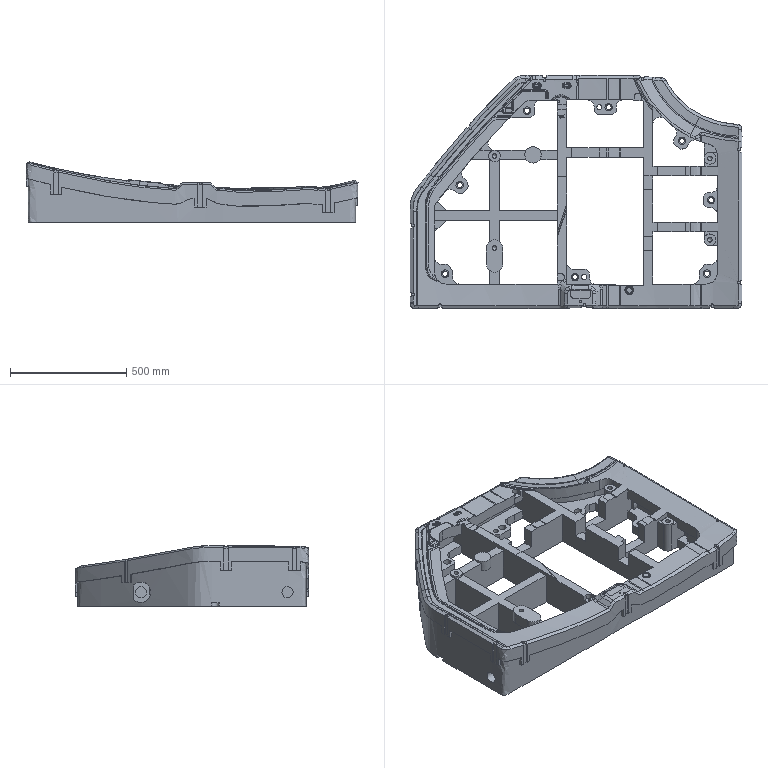Part | NX | features solid 2 | 1 solid | 711 faces | volume 63138841 mm3 | spline 387 | plane 240 | cylinder 80 | cone 4 | commonest cylinder face diameters 60 x19 10 x10 22 x10 32 x9 118 x6 190 x5